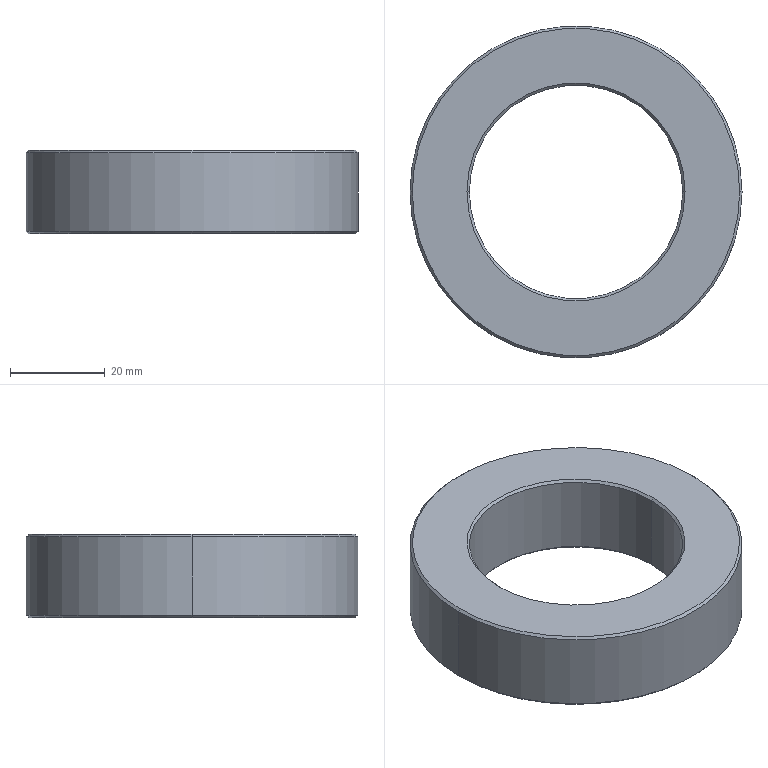Part | SolidWorks | features Chamfer 1, Extrusion 1 | 1 solid | 14 faces | box 70 x 70 x 17.5 mm | volume 39425 mm3 | cone 8 | cylinder 4 | plane 2 | commonest cylinder face diameters 45 x2 70 x2
STEP:
#1=CARTESIAN_POINT('',(34.5,0.,17.5));
#2=VERTEX_POINT('',#1);
#3=CARTESIAN_POINT('',(-34.5,0.,17.5));
#4=VERTEX_POINT('',#3);
#5=CARTESIAN_POINT('',(0.,0.,17.5));
#6=DIRECTION('',(0.,0.,1.));
#7=DIRECTION('',(1.,0.,0.));
#8=AXIS2_PLACEMENT_3D('',#5,#6,#7);
#9=CIRCLE('',#8,34.5);
#10=EDGE_CURVE('',#2,#4,#9,.T.);
#11=ORIENTED_EDGE('',*,*,#10,.F.);
#12=CARTESIAN_POINT('',(35.,0.,17.));
#13=VERTEX_POINT('',#12);
#14=CARTESIAN_POINT('',(34.5,0.,17.5));
#15=DIRECTION('',(0.7071,0.,-0.7071));
#16=VECTOR('',#15,1000.);
#17=LINE('',#14,#16);
#18=EDGE_CURVE('',#2,#13,#17,.T.);
#19=ORIENTED_EDGE('',*,*,#18,.T.);
#20=CARTESIAN_POINT('',(-35.,0.,17.));
#21=VERTEX_POINT('',#20);
#22=CARTESIAN_POINT('',(0.,0.,17.));
#23=DIRECTION('',(0.,0.,-1.));
#24=DIRECTION('',(1.,0.,0.));
#25=AXIS2_PLACEMENT_3D('',#22,#23,#24);
#26=CIRCLE('',#25,35.);
#27=EDGE_CURVE('',#21,#13,#26,.T.);
#28=ORIENTED_EDGE('',*,*,#27,.F.);
#29=CARTESIAN_POINT('',(-34.5,0.,17.5));
#30=DIRECTION('',(-0.7071,0.,-0.7071));
#31=VECTOR('',#30,1000.);
#32=LINE('',#29,#31);
#33=EDGE_CURVE('',#4,#21,#32,.T.);
#34=ORIENTED_EDGE('',*,*,#33,.F.);
#35=EDGE_LOOP('',(#11,#19,#28,#34));
#36=FACE_OUTER_BOUND('',#35,.T.);
#37=CARTESIAN_POINT('',(0.,0.,17.5));
#38=DIRECTION('',(0.,0.,-1.));
#39=DIRECTION('',(-1.,0.,0.));
#40=AXIS2_PLACEMENT_3D('',#37,#38,#39);
#41=CONICAL_SURFACE('',#40,34.5,0.7854);
#42=ADVANCED_FACE('',(#36),#41,.T.);
#43=CARTESIAN_POINT('',(-22.5,0.,17.));
#44=VERTEX_POINT('',#43);
#45=CARTESIAN_POINT('',(22.5,0.,17.));
#46=VERTEX_POINT('',#45);
#47=CARTESIAN_POINT('',(0.,0.,17.));
#48=DIRECTION('',(0.,0.,1.));
#49=DIRECTION('',(1.,0.,0.));
#50=AXIS2_PLACEMENT_3D('',#47,#48,#49);
#51=CIRCLE('',#50,22.5);
#52=EDGE_CURVE('',#44,#46,#51,.T.);
#53=ORIENTED_EDGE('',*,*,#52,.F.);
#54=CARTESIAN_POINT('',(-23.,0.,17.5));
#55=VERTEX_POINT('',#54);
#56=CARTESIAN_POINT('',(-22.5,0.,17.));
#57=DIRECTION('',(-0.7071,0.,0.7071));
#58=VECTOR('',#57,1000.);
#59=LINE('',#56,#58);
#60=EDGE_CURVE('',#44,#55,#59,.T.);
#61=ORIENTED_EDGE('',*,*,#60,.T.);
#62=CARTESIAN_POINT('',(23.,0.,17.5));
#63=VERTEX_POINT('',#62);
#64=CARTESIAN_POINT('',(0.,0.,17.5));
#65=DIRECTION('',(0.,0.,-1.));
#66=DIRECTION('',(1.,0.,0.));
#67=AXIS2_PLACEMENT_3D('',#64,#65,#66);
#68=CIRCLE('',#67,23.);
#69=EDGE_CURVE('',#63,#55,#68,.T.);
#70=ORIENTED_EDGE('',*,*,#69,.F.);
#71=CARTESIAN_POINT('',(22.5,0.,17.));
#72=DIRECTION('',(0.7071,0.,0.7071));
#73=VECTOR('',#72,1000.);
#74=LINE('',#71,#73);
#75=EDGE_CURVE('',#46,#63,#74,.T.);
#76=ORIENTED_EDGE('',*,*,#75,.F.);
#77=EDGE_LOOP('',(#53,#61,#70,#76));
#78=FACE_OUTER_BOUND('',#77,.T.);
#79=CARTESIAN_POINT('',(0.,0.,17.));
#80=DIRECTION('',(0.,0.,1.));
#81=DIRECTION('',(1.,0.,0.));
#82=AXIS2_PLACEMENT_3D('',#79,#80,#81);
#83=CONICAL_SURFACE('',#82,22.5,0.7854);
#84=ADVANCED_FACE('',(#78),#83,.F.);
#85=CARTESIAN_POINT('',(-34.5,0.,0.));
#86=VERTEX_POINT('',#85);
#87=CARTESIAN_POINT('',(34.5,0.,0.));
#88=VERTEX_POINT('',#87);
#89=CARTESIAN_POINT('',(0.,0.,0.));
#90=DIRECTION('',(0.,0.,-1.));
#91=DIRECTION('',(1.,0.,0.));
#92=AXIS2_PLACEMENT_3D('',#89,#90,#91);
#93=CIRCLE('',#92,34.5);
#94=EDGE_CURVE('',#86,#88,#93,.T.);
#95=ORIENTED_EDGE('',*,*,#94,.F.);
#96=CARTESIAN_POINT('',(-35.,0.,0.5));
#97=VERTEX_POINT('',#96);
#98=CARTESIAN_POINT('',(-35.,0.,0.5));
#99=DIRECTION('',(-0.7071,0.,0.7071));
#100=VECTOR('',#99,1000.);
#101=LINE('',#98,#100);
#102=EDGE_CURVE('',#86,#97,#101,.T.);
#103=ORIENTED_EDGE('',*,*,#102,.T.);
#104=CARTESIAN_POINT('',(35.,0.,0.5));
#105=VERTEX_POINT('',#104);
#106=CARTESIAN_POINT('',(0.,0.,0.5));
#107=DIRECTION('',(0.,0.,1.));
#108=DIRECTION('',(1.,0.,0.));
#109=AXIS2_PLACEMENT_3D('',#106,#107,#108);
#110=CIRCLE('',#109,35.);
#111=EDGE_CURVE('',#105,#97,#110,.T.);
#112=ORIENTED_EDGE('',*,*,#111,.F.);
#113=CARTESIAN_POINT('',(35.,0.,0.5));
#114=DIRECTION('',(0.7071,0.,0.7071));
#115=VECTOR('',#114,1000.);
#116=LINE('',#113,#115);
#117=EDGE_CURVE('',#88,#105,#116,.T.);
#118=ORIENTED_EDGE('',*,*,#117,.F.);
#119=EDGE_LOOP('',(#95,#103,#112,#118));
#120=FACE_OUTER_BOUND('',#119,.T.);
#121=CARTESIAN_POINT('',(0.,0.,0.5));
#122=DIRECTION('',(0.,0.,1.));
#123=DIRECTION('',(1.,0.,0.));
#124=AXIS2_PLACEMENT_3D('',#121,#122,#123);
#125=CONICAL_SURFACE('',#124,35.,0.7854);
#126=ADVANCED_FACE('',(#120),#125,.T.);
#127=CARTESIAN_POINT('',(22.5,0.,0.5));
#128=VERTEX_POINT('',#127);
#129=CARTESIAN_POINT('',(-22.5,0.,0.5));
#130=VERTEX_POINT('',#129);
#131=CARTESIAN_POINT('',(0.,0.,0.5));
#132=DIRECTION('',(0.,0.,-1.));
#133=DIRECTION('',(1.,0.,0.));
#134=AXIS2_PLACEMENT_3D('',#131,#132,#133);
#135=CIRCLE('',#134,22.5);
#136=EDGE_CURVE('',#128,#130,#135,.T.);
#137=ORIENTED_EDGE('',*,*,#136,.F.);
#138=CARTESIAN_POINT('',(23.,0.,0.));
#139=VERTEX_POINT('',#138);
#140=CARTESIAN_POINT('',(23.,0.,0.));
#141=DIRECTION('',(0.7071,0.,-0.7071));
#142=VECTOR('',#141,1000.);
#143=LINE('',#140,#142);
#144=EDGE_CURVE('',#128,#139,#143,.T.);
#145=ORIENTED_EDGE('',*,*,#144,.T.);
#146=CARTESIAN_POINT('',(-23.,0.,0.));
#147=VERTEX_POINT('',#146);
#148=CARTESIAN_POINT('',(0.,0.,0.));
#149=DIRECTION('',(0.,0.,1.));
#150=DIRECTION('',(1.,0.,0.));
#151=AXIS2_PLACEMENT_3D('',#148,#149,#150);
#152=CIRCLE('',#151,23.);
#153=EDGE_CURVE('',#147,#139,#152,.T.);
#154=ORIENTED_EDGE('',*,*,#153,.F.);
#155=CARTESIAN_POINT('',(-23.,0.,0.));
#156=DIRECTION('',(-0.7071,0.,-0.7071));
#157=VECTOR('',#156,1000.);
#158=LINE('',#155,#157);
#159=EDGE_CURVE('',#130,#147,#158,.T.);
#160=ORIENTED_EDGE('',*,*,#159,.F.);
#161=EDGE_LOOP('',(#137,#145,#154,#160));
#162=FACE_OUTER_BOUND('',#161,.T.);
#163=CARTESIAN_POINT('',(0.,0.,0.));
#164=DIRECTION('',(0.,0.,-1.));
#165=DIRECTION('',(-1.,0.,0.));
#166=AXIS2_PLACEMENT_3D('',#163,#164,#165);
#167=CONICAL_SURFACE('',#166,23.,0.7854);
#168=ADVANCED_FACE('',(#162),#167,.F.);
#169=ORIENTED_EDGE('',*,*,#52,.T.);
#170=CARTESIAN_POINT('',(22.5,0.,17.5));
#171=DIRECTION('',(0.,0.,-1.));
#172=VECTOR('',#171,1000.);
#173=LINE('',#170,#172);
#174=EDGE_CURVE('',#46,#128,#173,.T.);
#175=ORIENTED_EDGE('',*,*,#174,.T.);
#176=ORIENTED_EDGE('',*,*,#136,.T.);
#177=CARTESIAN_POINT('',(-22.5,0.,17.5));
#178=DIRECTION('',(0.,0.,-1.));
#179=VECTOR('',#178,1000.);
#180=LINE('',#177,#179);
#181=EDGE_CURVE('',#44,#130,#180,.T.);
#182=ORIENTED_EDGE('',*,*,#181,.F.);
#183=EDGE_LOOP('',(#169,#175,#176,#182));
#184=FACE_OUTER_BOUND('',#183,.T.);
#185=CARTESIAN_POINT('',(0.,0.,17.5));
#186=DIRECTION('',(0.,0.,-1.));
#187=DIRECTION('',(-1.,0.,0.));
#188=AXIS2_PLACEMENT_3D('',#185,#186,#187);
#189=CYLINDRICAL_SURFACE('',#188,22.5);
#190=ADVANCED_FACE('',(#184),#189,.F.);
#191=ORIENTED_EDGE('',*,*,#27,.T.);
#192=CARTESIAN_POINT('',(35.,0.,17.5));
#193=DIRECTION('',(0.,0.,-1.));
#194=VECTOR('',#193,1000.);
#195=LINE('',#192,#194);
#196=EDGE_CURVE('',#13,#105,#195,.T.);
#197=ORIENTED_EDGE('',*,*,#196,.T.);
#198=ORIENTED_EDGE('',*,*,#111,.T.);
#199=CARTESIAN_POINT('',(-35.,0.,17.5));
#200=DIRECTION('',(0.,0.,-1.));
#201=VECTOR('',#200,1000.);
#202=LINE('',#199,#201);
#203=EDGE_CURVE('',#21,#97,#202,.T.);
#204=ORIENTED_EDGE('',*,*,#203,.F.);
#205=EDGE_LOOP('',(#191,#197,#198,#204));
#206=FACE_OUTER_BOUND('',#205,.T.);
#207=CARTESIAN_POINT('',(0.,0.,17.5));
#208=DIRECTION('',(0.,0.,-1.));
#209=DIRECTION('',(-1.,0.,0.));
#210=AXIS2_PLACEMENT_3D('',#207,#208,#209);
#211=CYLINDRICAL_SURFACE('',#210,35.);
#212=ADVANCED_FACE('',(#206),#211,.T.);
#213=ORIENTED_EDGE('',*,*,#69,.T.);
#214=CARTESIAN_POINT('',(0.,0.,17.5));
#215=DIRECTION('',(0.,0.,-1.));
#216=DIRECTION('',(1.,0.,0.));
#217=AXIS2_PLACEMENT_3D('',#214,#215,#216);
#218=CIRCLE('',#217,23.);
#219=EDGE_CURVE('',#55,#63,#218,.T.);
#220=ORIENTED_EDGE('',*,*,#219,.T.);
#221=EDGE_LOOP('',(#213,#220));
#222=FACE_BOUND('',#221,.T.);
#223=CARTESIAN_POINT('',(0.,0.,17.5));
#224=DIRECTION('',(0.,0.,1.));
#225=DIRECTION('',(1.,0.,0.));
#226=AXIS2_PLACEMENT_3D('',#223,#224,#225);
#227=CIRCLE('',#226,34.5);
#228=EDGE_CURVE('',#4,#2,#227,.T.);
#229=ORIENTED_EDGE('',*,*,#228,.T.);
#230=ORIENTED_EDGE('',*,*,#10,.T.);
#231=EDGE_LOOP('',(#229,#230));
#232=FACE_OUTER_BOUND('',#231,.T.);
#233=CARTESIAN_POINT('',(0.,0.,17.5));
#234=DIRECTION('',(0.,0.,1.));
#235=DIRECTION('',(1.,0.,0.));
#236=AXIS2_PLACEMENT_3D('',#233,#234,#235);
#237=PLANE('',#236);
#238=ADVANCED_FACE('',(#222,#232),#237,.T.);
#239=ORIENTED_EDGE('',*,*,#153,.T.);
#240=CARTESIAN_POINT('',(0.,0.,0.));
#241=DIRECTION('',(0.,0.,1.));
#242=DIRECTION('',(1.,0.,0.));
#243=AXIS2_PLACEMENT_3D('',#240,#241,#242);
#244=CIRCLE('',#243,23.);
#245=EDGE_CURVE('',#139,#147,#244,.T.);
#246=ORIENTED_EDGE('',*,*,#245,.T.);
#247=EDGE_LOOP('',(#239,#246));
#248=FACE_BOUND('',#247,.T.);
#249=CARTESIAN_POINT('',(0.,0.,0.));
#250=DIRECTION('',(0.,0.,-1.));
#251=DIRECTION('',(1.,0.,0.));
#252=AXIS2_PLACEMENT_3D('',#249,#250,#251);
#253=CIRCLE('',#252,34.5);
#254=EDGE_CURVE('',#88,#86,#253,.T.);
#255=ORIENTED_EDGE('',*,*,#254,.T.);
#256=ORIENTED_EDGE('',*,*,#94,.T.);
#257=EDGE_LOOP('',(#255,#256));
#258=FACE_OUTER_BOUND('',#257,.T.);
#259=CARTESIAN_POINT('',(0.,0.,0.));
#260=DIRECTION('',(0.,0.,1.));
#261=DIRECTION('',(1.,0.,0.));
#262=AXIS2_PLACEMENT_3D('',#259,#260,#261);
#263=PLANE('',#262);
#264=ADVANCED_FACE('',(#248,#258),#263,.F.);
#265=ORIENTED_EDGE('',*,*,#196,.F.);
#266=CARTESIAN_POINT('',(0.,0.,17.));
#267=DIRECTION('',(0.,0.,-1.));
#268=DIRECTION('',(1.,0.,0.));
#269=AXIS2_PLACEMENT_3D('',#266,#267,#268);
#270=CIRCLE('',#269,35.);
#271=EDGE_CURVE('',#13,#21,#270,.T.);
#272=ORIENTED_EDGE('',*,*,#271,.T.);
#273=ORIENTED_EDGE('',*,*,#203,.T.);
#274=CARTESIAN_POINT('',(0.,0.,0.5));
#275=DIRECTION('',(0.,0.,1.));
#276=DIRECTION('',(1.,0.,0.));
#277=AXIS2_PLACEMENT_3D('',#274,#275,#276);
#278=CIRCLE('',#277,35.);
#279=EDGE_CURVE('',#97,#105,#278,.T.);
#280=ORIENTED_EDGE('',*,*,#279,.T.);
#281=EDGE_LOOP('',(#265,#272,#273,#280));
#282=FACE_OUTER_BOUND('',#281,.T.);
#283=CARTESIAN_POINT('',(0.,0.,17.5));
#284=DIRECTION('',(0.,0.,-1.));
#285=DIRECTION('',(-1.,0.,0.));
#286=AXIS2_PLACEMENT_3D('',#283,#284,#285);
#287=CYLINDRICAL_SURFACE('',#286,35.);
#288=ADVANCED_FACE('',(#282),#287,.T.);
#289=ORIENTED_EDGE('',*,*,#174,.F.);
#290=CARTESIAN_POINT('',(0.,0.,17.));
#291=DIRECTION('',(0.,0.,1.));
#292=DIRECTION('',(1.,0.,0.));
#293=AXIS2_PLACEMENT_3D('',#290,#291,#292);
#294=CIRCLE('',#293,22.5);
#295=EDGE_CURVE('',#46,#44,#294,.T.);
#296=ORIENTED_EDGE('',*,*,#295,.T.);
#297=ORIENTED_EDGE('',*,*,#181,.T.);
#298=CARTESIAN_POINT('',(0.,0.,0.5));
#299=DIRECTION('',(0.,0.,-1.));
#300=DIRECTION('',(1.,0.,0.));
#301=AXIS2_PLACEMENT_3D('',#298,#299,#300);
#302=CIRCLE('',#301,22.5);
#303=EDGE_CURVE('',#130,#128,#302,.T.);
#304=ORIENTED_EDGE('',*,*,#303,.T.);
#305=EDGE_LOOP('',(#289,#296,#297,#304));
#306=FACE_OUTER_BOUND('',#305,.T.);
#307=CARTESIAN_POINT('',(0.,0.,17.5));
#308=DIRECTION('',(0.,0.,-1.));
#309=DIRECTION('',(-1.,0.,0.));
#310=AXIS2_PLACEMENT_3D('',#307,#308,#309);
#311=CYLINDRICAL_SURFACE('',#310,22.5);
#312=ADVANCED_FACE('',(#306),#311,.F.);
#313=ORIENTED_EDGE('',*,*,#144,.F.);
#314=ORIENTED_EDGE('',*,*,#303,.F.);
#315=ORIENTED_EDGE('',*,*,#159,.T.);
#316=ORIENTED_EDGE('',*,*,#245,.F.);
#317=EDGE_LOOP('',(#313,#314,#315,#316));
#318=FACE_OUTER_BOUND('',#317,.T.);
#319=CARTESIAN_POINT('',(0.,0.,0.));
#320=DIRECTION('',(0.,0.,-1.));
#321=DIRECTION('',(-1.,0.,0.));
#322=AXIS2_PLACEMENT_3D('',#319,#320,#321);
#323=CONICAL_SURFACE('',#322,23.,0.7854);
#324=ADVANCED_FACE('',(#318),#323,.F.);
#325=ORIENTED_EDGE('',*,*,#102,.F.);
#326=ORIENTED_EDGE('',*,*,#254,.F.);
#327=ORIENTED_EDGE('',*,*,#117,.T.);
#328=ORIENTED_EDGE('',*,*,#279,.F.);
#329=EDGE_LOOP('',(#325,#326,#327,#328));
#330=FACE_OUTER_BOUND('',#329,.T.);
#331=CARTESIAN_POINT('',(0.,0.,0.5));
#332=DIRECTION('',(0.,0.,1.));
#333=DIRECTION('',(1.,0.,0.));
#334=AXIS2_PLACEMENT_3D('',#331,#332,#333);
#335=CONICAL_SURFACE('',#334,35.,0.7854);
#336=ADVANCED_FACE('',(#330),#335,.T.);
#337=ORIENTED_EDGE('',*,*,#60,.F.);
#338=ORIENTED_EDGE('',*,*,#295,.F.);
#339=ORIENTED_EDGE('',*,*,#75,.T.);
#340=ORIENTED_EDGE('',*,*,#219,.F.);
#341=EDGE_LOOP('',(#337,#338,#339,#340));
#342=FACE_OUTER_BOUND('',#341,.T.);
#343=CARTESIAN_POINT('',(0.,0.,17.));
#344=DIRECTION('',(0.,0.,1.));
#345=DIRECTION('',(1.,0.,0.));
#346=AXIS2_PLACEMENT_3D('',#343,#344,#345);
#347=CONICAL_SURFACE('',#346,22.5,0.7854);
#348=ADVANCED_FACE('',(#342),#347,.F.);
#349=ORIENTED_EDGE('',*,*,#18,.F.);
#350=ORIENTED_EDGE('',*,*,#228,.F.);
#351=ORIENTED_EDGE('',*,*,#33,.T.);
#352=ORIENTED_EDGE('',*,*,#271,.F.);
#353=EDGE_LOOP('',(#349,#350,#351,#352));
#354=FACE_OUTER_BOUND('',#353,.T.);
#355=CARTESIAN_POINT('',(0.,0.,17.5));
#356=DIRECTION('',(0.,0.,-1.));
#357=DIRECTION('',(-1.,0.,0.));
#358=AXIS2_PLACEMENT_3D('',#355,#356,#357);
#359=CONICAL_SURFACE('',#358,34.5,0.7854);
#360=ADVANCED_FACE('',(#354),#359,.T.);
#361=CLOSED_SHELL('',(#42,#84,#126,#168,#190,#212,#238,#264,#288,#312,#324,#336,#348,#360));
#362=MANIFOLD_SOLID_BREP('',#361);
#363=CARTESIAN_POINT('',(0.,0.,0.));
#364=DIRECTION('',(0.,0.,1.));
#365=DIRECTION('',(1.,0.,0.));
#366=AXIS2_PLACEMENT_3D('',#363,#364,#365);
#367=(LENGTH_UNIT()NAMED_UNIT(*)SI_UNIT(.MILLI.,.METRE.));
#368=UNCERTAINTY_MEASURE_WITH_UNIT(LENGTH_MEASURE(0.00001),#367,'','');
#369=(NAMED_UNIT(*)PLANE_ANGLE_UNIT()SI_UNIT($,.RADIAN.));
#370=(NAMED_UNIT(*)SI_UNIT($,.STERADIAN.)SOLID_ANGLE_UNIT());
#371=(GEOMETRIC_REPRESENTATION_CONTEXT(3)GLOBAL_UNCERTAINTY_ASSIGNED_CONTEXT((#368))GLOBAL_UNIT_ASSIGNED_CONTEXT((#367,#369,#370))REPRESENTATION_CONTEXT('',''));
#372=ADVANCED_BREP_SHAPE_REPRESENTATION('',(#362,#366),#371);